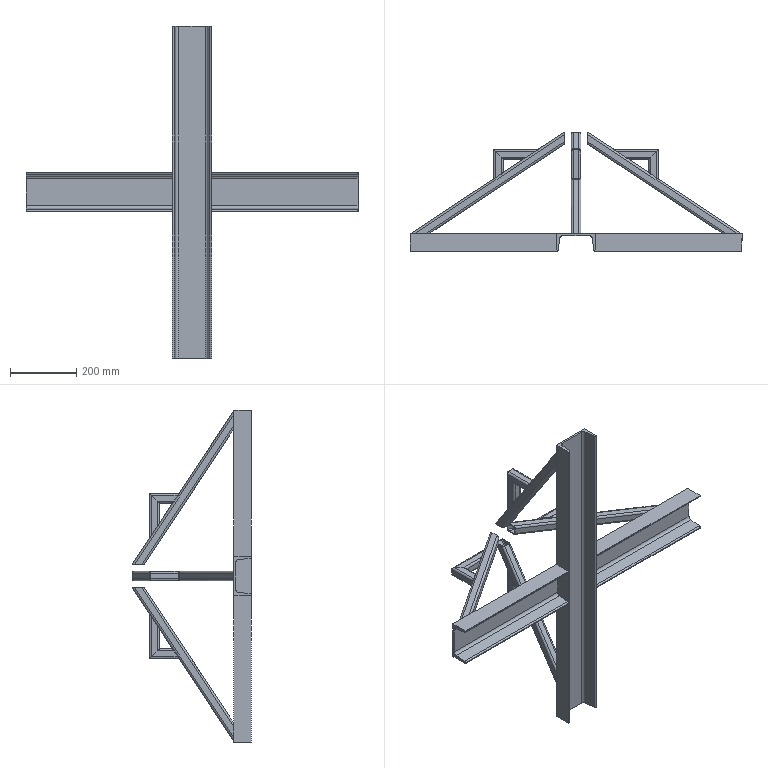Part | SolidWorks | features WeldMemberFeat 3, WeldCornerFeat 2, CirPattern 1, ICE 1, RefAxis 1, WeldmentFeature 1 | 15 solids | 262 faces | box 1000 x 358.035 x 1000 mm | volume 3764045 mm3 | plane 154 | cylinder 108 | commonest cylinder face diameters 5.6 x48 12 x48 9 x6 18 x6